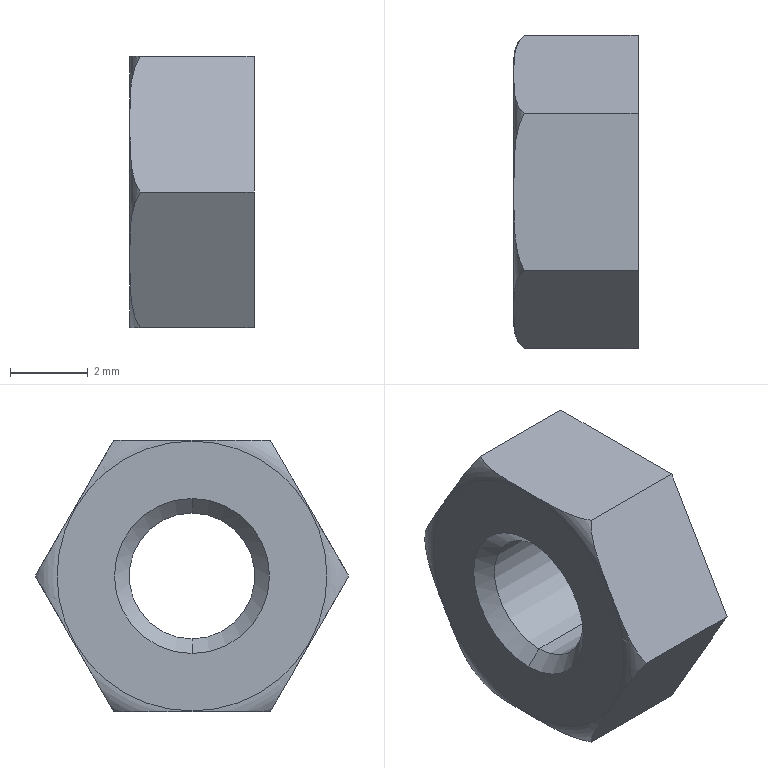Part | SolidWorks | features RefAxis 3, 3DProfileFeature 1, ICE 1, RevCut 1, Revolution 1 | 1 solid | 16 faces | box 3.2 x 8.083 x 7 mm | volume 107.662 mm3 | plane 8 | cone 4 | cylinder 2 | torus 2 | commonest cylinder face diameters 3.242 x2
STEP:
#1=CARTESIAN_POINT('',(1.221,0.,-1.621));
#2=VERTEX_POINT('',#1);
#3=CARTESIAN_POINT('',(1.221,0.,1.621));
#4=VERTEX_POINT('',#3);
#5=CARTESIAN_POINT('',(1.221,0.,0.));
#6=DIRECTION('',(-1.,0.,0.));
#7=DIRECTION('',(0.,0.,1.));
#8=AXIS2_PLACEMENT_3D('',#5,#6,#7);
#9=CIRCLE('',#8,1.621);
#10=EDGE_CURVE('',#2,#4,#9,.T.);
#11=ORIENTED_EDGE('',*,*,#10,.T.);
#12=CARTESIAN_POINT('',(1.6,0.,2.));
#13=VERTEX_POINT('',#12);
#14=CARTESIAN_POINT('',(1.6,0.,2.));
#15=DIRECTION('',(0.7071,0.,0.7071));
#16=VECTOR('',#15,1000.);
#17=LINE('',#14,#16);
#18=EDGE_CURVE('',#4,#13,#17,.T.);
#19=ORIENTED_EDGE('',*,*,#18,.T.);
#20=CARTESIAN_POINT('',(1.6,0.,-2.));
#21=VERTEX_POINT('',#20);
#22=CARTESIAN_POINT('',(1.6,0.,0.));
#23=DIRECTION('',(-1.,0.,0.));
#24=DIRECTION('',(0.,0.,1.));
#25=AXIS2_PLACEMENT_3D('',#22,#23,#24);
#26=CIRCLE('',#25,2.);
#27=EDGE_CURVE('',#21,#13,#26,.T.);
#28=ORIENTED_EDGE('',*,*,#27,.F.);
#29=CARTESIAN_POINT('',(1.6,0.,-2.));
#30=DIRECTION('',(0.7071,0.,-0.7071));
#31=VECTOR('',#30,1000.);
#32=LINE('',#29,#31);
#33=EDGE_CURVE('',#2,#21,#32,.T.);
#34=ORIENTED_EDGE('',*,*,#33,.F.);
#35=EDGE_LOOP('',(#11,#19,#28,#34));
#36=FACE_OUTER_BOUND('',#35,.T.);
#37=CARTESIAN_POINT('',(1.6,0.,0.));
#38=DIRECTION('',(1.,0.,0.));
#39=DIRECTION('',(0.,0.,-1.));
#40=AXIS2_PLACEMENT_3D('',#37,#38,#39);
#41=CONICAL_SURFACE('',#40,2.,0.7854);
#42=ADVANCED_FACE('',(#36),#41,.F.);
#43=ORIENTED_EDGE('',*,*,#10,.F.);
#44=CARTESIAN_POINT('',(-1.221,0.,-1.621));
#45=VERTEX_POINT('',#44);
#46=CARTESIAN_POINT('',(1.6,0.,-1.621));
#47=DIRECTION('',(-1.,0.,0.));
#48=VECTOR('',#47,1000.);
#49=LINE('',#46,#48);
#50=EDGE_CURVE('',#2,#45,#49,.T.);
#51=ORIENTED_EDGE('',*,*,#50,.T.);
#52=CARTESIAN_POINT('',(-1.221,0.,1.621));
#53=VERTEX_POINT('',#52);
#54=CARTESIAN_POINT('',(-1.221,0.,0.));
#55=DIRECTION('',(-1.,0.,0.));
#56=DIRECTION('',(0.,0.,1.));
#57=AXIS2_PLACEMENT_3D('',#54,#55,#56);
#58=CIRCLE('',#57,1.621);
#59=EDGE_CURVE('',#45,#53,#58,.T.);
#60=ORIENTED_EDGE('',*,*,#59,.T.);
#61=CARTESIAN_POINT('',(1.6,0.,1.621));
#62=DIRECTION('',(-1.,0.,0.));
#63=VECTOR('',#62,1000.);
#64=LINE('',#61,#63);
#65=EDGE_CURVE('',#4,#53,#64,.T.);
#66=ORIENTED_EDGE('',*,*,#65,.F.);
#67=EDGE_LOOP('',(#43,#51,#60,#66));
#68=FACE_OUTER_BOUND('',#67,.T.);
#69=CARTESIAN_POINT('',(1.6,0.,0.));
#70=DIRECTION('',(-1.,0.,0.));
#71=DIRECTION('',(0.,0.,1.));
#72=AXIS2_PLACEMENT_3D('',#69,#70,#71);
#73=CYLINDRICAL_SURFACE('',#72,1.621);
#74=ADVANCED_FACE('',(#68),#73,.F.);
#75=ORIENTED_EDGE('',*,*,#59,.F.);
#76=CARTESIAN_POINT('',(-1.6,0.,-2.));
#77=VERTEX_POINT('',#76);
#78=CARTESIAN_POINT('',(-1.221,0.,-1.621));
#79=DIRECTION('',(-0.7071,0.,-0.7071));
#80=VECTOR('',#79,1000.);
#81=LINE('',#78,#80);
#82=EDGE_CURVE('',#45,#77,#81,.T.);
#83=ORIENTED_EDGE('',*,*,#82,.T.);
#84=CARTESIAN_POINT('',(-1.6,0.,2.));
#85=VERTEX_POINT('',#84);
#86=CARTESIAN_POINT('',(-1.6,0.,0.));
#87=DIRECTION('',(-1.,0.,0.));
#88=DIRECTION('',(0.,0.,1.));
#89=AXIS2_PLACEMENT_3D('',#86,#87,#88);
#90=CIRCLE('',#89,2.);
#91=EDGE_CURVE('',#77,#85,#90,.T.);
#92=ORIENTED_EDGE('',*,*,#91,.T.);
#93=CARTESIAN_POINT('',(-1.221,0.,1.621));
#94=DIRECTION('',(-0.7071,0.,0.7071));
#95=VECTOR('',#94,1000.);
#96=LINE('',#93,#95);
#97=EDGE_CURVE('',#53,#85,#96,.T.);
#98=ORIENTED_EDGE('',*,*,#97,.F.);
#99=EDGE_LOOP('',(#75,#83,#92,#98));
#100=FACE_OUTER_BOUND('',#99,.T.);
#101=CARTESIAN_POINT('',(-1.221,0.,0.));
#102=DIRECTION('',(-1.,0.,0.));
#103=DIRECTION('',(0.,0.,1.));
#104=AXIS2_PLACEMENT_3D('',#101,#102,#103);
#105=CONICAL_SURFACE('',#104,1.621,0.7854);
#106=ADVANCED_FACE('',(#100),#105,.F.);
#107=CARTESIAN_POINT('',(-1.6,0.,-3.5));
#108=VERTEX_POINT('',#107);
#109=CARTESIAN_POINT('',(-1.331,2.021,-3.5));
#110=VERTEX_POINT('',#109);
#111=CARTESIAN_POINT('',(-1.6,0.,-3.5));
#112=CARTESIAN_POINT('',(-1.6,0.3431,-3.5));
#113=CARTESIAN_POINT('',(-1.603,0.6864,-3.5));
#114=CARTESIAN_POINT('',(-1.569,1.2,-3.5));
#115=CARTESIAN_POINT('',(-1.549,1.371,-3.5));
#116=CARTESIAN_POINT('',(-1.494,1.624,-3.5));
#117=CARTESIAN_POINT('',(-1.472,1.706,-3.5));
#118=CARTESIAN_POINT('',(-1.413,1.868,-3.5));
#119=CARTESIAN_POINT('',(-1.376,1.948,-3.5));
#120=CARTESIAN_POINT('',(-1.331,2.021,-3.5));
#121=B_SPLINE_CURVE_WITH_KNOTS('',3,(#111,#112,#113,#114,#115,#116,#117,#118,#119,#120),.UNSPECIFIED.,.F.,.F.,(4,2,2,2,4),(0.,0.001028,0.001542,0.001799,0.002057),.UNSPECIFIED.);
#122=EDGE_CURVE('',#108,#110,#121,.T.);
#123=ORIENTED_EDGE('',*,*,#122,.F.);
#124=CARTESIAN_POINT('',(-1.6,0.,-3.48));
#125=VERTEX_POINT('',#124);
#126=CARTESIAN_POINT('',(-0.88,0.,-3.48));
#127=DIRECTION('',(0.,1.,0.));
#128=DIRECTION('',(0.,0.,1.));
#129=AXIS2_PLACEMENT_3D('',#126,#127,#128);
#130=CIRCLE('',#129,0.72);
#131=EDGE_CURVE('',#108,#125,#130,.T.);
#132=ORIENTED_EDGE('',*,*,#131,.T.);
#133=CARTESIAN_POINT('',(-1.6,0.,3.48));
#134=VERTEX_POINT('',#133);
#135=CARTESIAN_POINT('',(-1.6,0.,0.));
#136=DIRECTION('',(-1.,0.,0.));
#137=DIRECTION('',(0.,0.,1.));
#138=AXIS2_PLACEMENT_3D('',#135,#136,#137);
#139=CIRCLE('',#138,3.48);
#140=EDGE_CURVE('',#134,#125,#139,.T.);
#141=ORIENTED_EDGE('',*,*,#140,.F.);
#142=CARTESIAN_POINT('',(-1.6,0.,3.5));
#143=VERTEX_POINT('',#142);
#144=CARTESIAN_POINT('',(-0.88,0.,3.48));
#145=DIRECTION('',(0.,-1.,0.));
#146=DIRECTION('',(0.,0.,-1.));
#147=AXIS2_PLACEMENT_3D('',#144,#145,#146);
#148=CIRCLE('',#147,0.72);
#149=EDGE_CURVE('',#143,#134,#148,.T.);
#150=ORIENTED_EDGE('',*,*,#149,.F.);
#151=CARTESIAN_POINT('',(-1.331,2.021,3.5));
#152=VERTEX_POINT('',#151);
#153=CARTESIAN_POINT('',(-1.331,2.021,3.5));
#154=CARTESIAN_POINT('',(-1.422,1.874,3.5));
#155=CARTESIAN_POINT('',(-1.476,1.706,3.5));
#156=CARTESIAN_POINT('',(-1.549,1.372,3.5));
#157=CARTESIAN_POINT('',(-1.568,1.202,3.5));
#158=CARTESIAN_POINT('',(-1.592,0.8597,3.5));
#159=CARTESIAN_POINT('',(-1.596,0.6875,3.5));
#160=CARTESIAN_POINT('',(-1.6,0.3438,3.5));
#161=CARTESIAN_POINT('',(-1.6,0.1724,3.5));
#162=CARTESIAN_POINT('',(-1.6,0.,3.5));
#163=B_SPLINE_CURVE_WITH_KNOTS('',3,(#153,#154,#155,#156,#157,#158,#159,#160,#161,#162),.UNSPECIFIED.,.F.,.F.,(4,2,2,2,4),(0.008439,0.008956,0.009473,0.009989,0.01051),.UNSPECIFIED.);
#164=EDGE_CURVE('',#152,#143,#163,.T.);
#165=ORIENTED_EDGE('',*,*,#164,.F.);
#166=CARTESIAN_POINT('',(-1.331,4.041,0.));
#167=VERTEX_POINT('',#166);
#168=CARTESIAN_POINT('',(-1.331,4.041,0.));
#169=CARTESIAN_POINT('',(-1.424,3.967,0.1292));
#170=CARTESIAN_POINT('',(-1.477,3.884,0.2733));
#171=CARTESIAN_POINT('',(-1.55,3.714,0.5673));
#172=CARTESIAN_POINT('',(-1.569,3.629,0.7151));
#173=CARTESIAN_POINT('',(-1.603,3.372,1.159));
#174=CARTESIAN_POINT('',(-1.6,3.2,1.457));
#175=CARTESIAN_POINT('',(-1.6,2.857,2.051));
#176=CARTESIAN_POINT('',(-1.603,2.686,2.348));
#177=CARTESIAN_POINT('',(-1.568,2.429,2.793));
#178=CARTESIAN_POINT('',(-1.549,2.343,2.941));
#179=CARTESIAN_POINT('',(-1.475,2.176,3.231));
#180=CARTESIAN_POINT('',(-1.423,2.095,3.372));
#181=CARTESIAN_POINT('',(-1.331,2.021,3.5));
#182=B_SPLINE_CURVE_WITH_KNOTS('',3,(#168,#169,#170,#171,#172,#173,#174,#175,#176,#177,#178,#179,#180,#181),.UNSPECIFIED.,.F.,.F.,(4,2,2,2,2,2,4),(0.000000268,0.0005191,0.001038,0.002076,0.003113,0.003632,0.004151),.UNSPECIFIED.);
#183=EDGE_CURVE('',#167,#152,#182,.T.);
#184=ORIENTED_EDGE('',*,*,#183,.F.);
#185=CARTESIAN_POINT('',(-1.331,2.021,-3.5));
#186=CARTESIAN_POINT('',(-1.424,2.095,-3.371));
#187=CARTESIAN_POINT('',(-1.477,2.179,-3.227));
#188=CARTESIAN_POINT('',(-1.55,2.348,-2.933));
#189=CARTESIAN_POINT('',(-1.569,2.434,-2.785));
#190=CARTESIAN_POINT('',(-1.603,2.69,-2.341));
#191=CARTESIAN_POINT('',(-1.6,2.862,-2.043));
#192=CARTESIAN_POINT('',(-1.6,3.205,-1.449));
#193=CARTESIAN_POINT('',(-1.603,3.377,-1.152));
#194=CARTESIAN_POINT('',(-1.568,3.633,-0.7074));
#195=CARTESIAN_POINT('',(-1.549,3.719,-0.5586));
#196=CARTESIAN_POINT('',(-1.475,3.886,-0.2687));
#197=CARTESIAN_POINT('',(-1.423,3.967,-0.1283));
#198=CARTESIAN_POINT('',(-1.331,4.041,0.));
#199=B_SPLINE_CURVE_WITH_KNOTS('',3,(#185,#186,#187,#188,#189,#190,#191,#192,#193,#194,#195,#196,#197,#198),.UNSPECIFIED.,.F.,.F.,(4,2,2,2,2,2,4),(0.000000268,0.0005191,0.001038,0.002076,0.003113,0.003632,0.004151),.UNSPECIFIED.);
#200=EDGE_CURVE('',#110,#167,#199,.T.);
#201=ORIENTED_EDGE('',*,*,#200,.F.);
#202=EDGE_LOOP('',(#123,#132,#141,#150,#165,#184,#201));
#203=FACE_OUTER_BOUND('',#202,.T.);
#204=CARTESIAN_POINT('',(-0.88,0.,0.));
#205=DIRECTION('',(-1.,0.,0.));
#206=DIRECTION('',(0.,0.,1.));
#207=AXIS2_PLACEMENT_3D('',#204,#205,#206);
#208=TOROIDAL_SURFACE('',#207,3.48,0.72);
#209=ADVANCED_FACE('',(#203),#208,.T.);
#210=ORIENTED_EDGE('',*,*,#27,.T.);
#211=CARTESIAN_POINT('',(1.6,0.,0.));
#212=DIRECTION('',(-1.,0.,0.));
#213=DIRECTION('',(0.,0.,1.));
#214=AXIS2_PLACEMENT_3D('',#211,#212,#213);
#215=CIRCLE('',#214,2.);
#216=EDGE_CURVE('',#13,#21,#215,.T.);
#217=ORIENTED_EDGE('',*,*,#216,.T.);
#218=EDGE_LOOP('',(#210,#217));
#219=FACE_BOUND('',#218,.T.);
#220=CARTESIAN_POINT('',(1.6,4.041,0.));
#221=VERTEX_POINT('',#220);
#222=CARTESIAN_POINT('',(1.6,2.021,3.5));
#223=VERTEX_POINT('',#222);
#224=CARTESIAN_POINT('',(1.6,4.041,0.));
#225=DIRECTION('',(0.,-0.5,0.866));
#226=VECTOR('',#225,1000.);
#227=LINE('',#224,#226);
#228=EDGE_CURVE('',#221,#223,#227,.T.);
#229=ORIENTED_EDGE('',*,*,#228,.T.);
#230=CARTESIAN_POINT('',(1.6,-2.021,3.5));
#231=VERTEX_POINT('',#230);
#232=CARTESIAN_POINT('',(1.6,2.021,3.5));
#233=DIRECTION('',(0.,-1.,0.));
#234=VECTOR('',#233,1000.);
#235=LINE('',#232,#234);
#236=EDGE_CURVE('',#223,#231,#235,.T.);
#237=ORIENTED_EDGE('',*,*,#236,.T.);
#238=CARTESIAN_POINT('',(1.6,-4.041,0.));
#239=VERTEX_POINT('',#238);
#240=CARTESIAN_POINT('',(1.6,-2.021,3.5));
#241=DIRECTION('',(0.,-0.5,-0.866));
#242=VECTOR('',#241,1000.);
#243=LINE('',#240,#242);
#244=EDGE_CURVE('',#231,#239,#243,.T.);
#245=ORIENTED_EDGE('',*,*,#244,.T.);
#246=CARTESIAN_POINT('',(1.6,-2.021,-3.5));
#247=VERTEX_POINT('',#246);
#248=CARTESIAN_POINT('',(1.6,-4.041,0.));
#249=DIRECTION('',(0.,0.5,-0.866));
#250=VECTOR('',#249,1000.);
#251=LINE('',#248,#250);
#252=EDGE_CURVE('',#239,#247,#251,.T.);
#253=ORIENTED_EDGE('',*,*,#252,.T.);
#254=CARTESIAN_POINT('',(1.6,2.021,-3.5));
#255=VERTEX_POINT('',#254);
#256=CARTESIAN_POINT('',(1.6,-2.021,-3.5));
#257=DIRECTION('',(0.,1.,0.));
#258=VECTOR('',#257,1000.);
#259=LINE('',#256,#258);
#260=EDGE_CURVE('',#247,#255,#259,.T.);
#261=ORIENTED_EDGE('',*,*,#260,.T.);
#262=CARTESIAN_POINT('',(1.6,2.021,-3.5));
#263=DIRECTION('',(0.,0.5,0.866));
#264=VECTOR('',#263,1000.);
#265=LINE('',#262,#264);
#266=EDGE_CURVE('',#255,#221,#265,.T.);
#267=ORIENTED_EDGE('',*,*,#266,.T.);
#268=EDGE_LOOP('',(#229,#237,#245,#253,#261,#267));
#269=FACE_OUTER_BOUND('',#268,.T.);
#270=CARTESIAN_POINT('',(1.6,4.2,0.));
#271=DIRECTION('',(-1.,0.,0.));
#272=DIRECTION('',(0.,0.,1.));
#273=AXIS2_PLACEMENT_3D('',#270,#271,#272);
#274=PLANE('',#273);
#275=ADVANCED_FACE('',(#219,#269),#274,.F.);
#276=ORIENTED_EDGE('',*,*,#131,.F.);
#277=CARTESIAN_POINT('',(-1.331,-2.021,-3.5));
#278=VERTEX_POINT('',#277);
#279=CARTESIAN_POINT('',(-1.331,-2.021,-3.5));
#280=CARTESIAN_POINT('',(-1.422,-1.874,-3.5));
#281=CARTESIAN_POINT('',(-1.476,-1.706,-3.5));
#282=CARTESIAN_POINT('',(-1.549,-1.372,-3.5));
#283=CARTESIAN_POINT('',(-1.568,-1.202,-3.5));
#284=CARTESIAN_POINT('',(-1.592,-0.8597,-3.5));
#285=CARTESIAN_POINT('',(-1.596,-0.6875,-3.5));
#286=CARTESIAN_POINT('',(-1.6,-0.3438,-3.5));
#287=CARTESIAN_POINT('',(-1.6,-0.1724,-3.5));
#288=CARTESIAN_POINT('',(-1.6,0.,-3.5));
#289=B_SPLINE_CURVE_WITH_KNOTS('',3,(#279,#280,#281,#282,#283,#284,#285,#286,#287,#288),.UNSPECIFIED.,.F.,.F.,(4,2,2,2,4),(0.008439,0.008956,0.009473,0.009989,0.01051),.UNSPECIFIED.);
#290=EDGE_CURVE('',#278,#108,#289,.T.);
#291=ORIENTED_EDGE('',*,*,#290,.F.);
#292=CARTESIAN_POINT('',(-1.331,-4.041,0.));
#293=VERTEX_POINT('',#292);
#294=CARTESIAN_POINT('',(-1.331,-4.041,0.));
#295=CARTESIAN_POINT('',(-1.424,-3.967,-0.1292));
#296=CARTESIAN_POINT('',(-1.477,-3.884,-0.2733));
#297=CARTESIAN_POINT('',(-1.55,-3.714,-0.5673));
#298=CARTESIAN_POINT('',(-1.569,-3.629,-0.7151));
#299=CARTESIAN_POINT('',(-1.603,-3.372,-1.159));
#300=CARTESIAN_POINT('',(-1.6,-3.2,-1.457));
#301=CARTESIAN_POINT('',(-1.6,-2.857,-2.051));
#302=CARTESIAN_POINT('',(-1.603,-2.686,-2.348));
#303=CARTESIAN_POINT('',(-1.568,-2.429,-2.793));
#304=CARTESIAN_POINT('',(-1.549,-2.343,-2.941));
#305=CARTESIAN_POINT('',(-1.475,-2.176,-3.231));
#306=CARTESIAN_POINT('',(-1.423,-2.095,-3.372));
#307=CARTESIAN_POINT('',(-1.331,-2.021,-3.5));
#308=B_SPLINE_CURVE_WITH_KNOTS('',3,(#294,#295,#296,#297,#298,#299,#300,#301,#302,#303,#304,#305,#306,#307),.UNSPECIFIED.,.F.,.F.,(4,2,2,2,2,2,4),(0.000000268,0.0005191,0.001038,0.002076,0.003113,0.003632,0.004151),.UNSPECIFIED.);
#309=EDGE_CURVE('',#293,#278,#308,.T.);
#310=ORIENTED_EDGE('',*,*,#309,.F.);
#311=CARTESIAN_POINT('',(-1.331,-2.021,3.5));
#312=VERTEX_POINT('',#311);
#313=CARTESIAN_POINT('',(-1.331,-2.021,3.5));
#314=CARTESIAN_POINT('',(-1.424,-2.095,3.371));
#315=CARTESIAN_POINT('',(-1.477,-2.179,3.227));
#316=CARTESIAN_POINT('',(-1.55,-2.348,2.933));
#317=CARTESIAN_POINT('',(-1.569,-2.434,2.785));
#318=CARTESIAN_POINT('',(-1.603,-2.69,2.341));
#319=CARTESIAN_POINT('',(-1.6,-2.862,2.043));
#320=CARTESIAN_POINT('',(-1.6,-3.205,1.449));
#321=CARTESIAN_POINT('',(-1.603,-3.377,1.152));
#322=CARTESIAN_POINT('',(-1.568,-3.633,0.7074));
#323=CARTESIAN_POINT('',(-1.549,-3.719,0.5586));
#324=CARTESIAN_POINT('',(-1.475,-3.886,0.2687));
#325=CARTESIAN_POINT('',(-1.423,-3.967,0.1283));
#326=CARTESIAN_POINT('',(-1.331,-4.041,0.));
#327=B_SPLINE_CURVE_WITH_KNOTS('',3,(#313,#314,#315,#316,#317,#318,#319,#320,#321,#322,#323,#324,#325,#326),.UNSPECIFIED.,.F.,.F.,(4,2,2,2,2,2,4),(0.000000268,0.0005191,0.001038,0.002076,0.003113,0.003632,0.004151),.UNSPECIFIED.);
#328=EDGE_CURVE('',#312,#293,#327,.T.);
#329=ORIENTED_EDGE('',*,*,#328,.F.);
#330=CARTESIAN_POINT('',(-1.6,0.,3.5));
#331=CARTESIAN_POINT('',(-1.6,-0.3431,3.5));
#332=CARTESIAN_POINT('',(-1.603,-0.6864,3.5));
#333=CARTESIAN_POINT('',(-1.569,-1.2,3.5));
#334=CARTESIAN_POINT('',(-1.549,-1.371,3.5));
#335=CARTESIAN_POINT('',(-1.494,-1.624,3.5));
#336=CARTESIAN_POINT('',(-1.472,-1.706,3.5));
#337=CARTESIAN_POINT('',(-1.413,-1.868,3.5));
#338=CARTESIAN_POINT('',(-1.376,-1.948,3.5));
#339=CARTESIAN_POINT('',(-1.331,-2.021,3.5));
#340=B_SPLINE_CURVE_WITH_KNOTS('',3,(#330,#331,#332,#333,#334,#335,#336,#337,#338,#339),.UNSPECIFIED.,.F.,.F.,(4,2,2,2,4),(0.,0.001028,0.001542,0.001799,0.002057),.UNSPECIFIED.);
#341=EDGE_CURVE('',#143,#312,#340,.T.);
#342=ORIENTED_EDGE('',*,*,#341,.F.);
#343=ORIENTED_EDGE('',*,*,#149,.T.);
#344=CARTESIAN_POINT('',(-1.6,0.,0.));
#345=DIRECTION('',(-1.,0.,0.));
#346=DIRECTION('',(0.,0.,1.));
#347=AXIS2_PLACEMENT_3D('',#344,#345,#346);
#348=CIRCLE('',#347,3.48);
#349=EDGE_CURVE('',#125,#134,#348,.T.);
#350=ORIENTED_EDGE('',*,*,#349,.F.);
#351=EDGE_LOOP('',(#276,#291,#310,#329,#342,#343,#350));
#352=FACE_OUTER_BOUND('',#351,.T.);
#353=CARTESIAN_POINT('',(-0.88,0.,0.));
#354=DIRECTION('',(-1.,0.,0.));
#355=DIRECTION('',(0.,0.,1.));
#356=AXIS2_PLACEMENT_3D('',#353,#354,#355);
#357=TOROIDAL_SURFACE('',#356,3.48,0.72);
#358=ADVANCED_FACE('',(#352),#357,.T.);
#359=ORIENTED_EDGE('',*,*,#140,.T.);
#360=ORIENTED_EDGE('',*,*,#349,.T.);
#361=EDGE_LOOP('',(#359,#360));
#362=FACE_OUTER_BOUND('',#361,.T.);
#363=CARTESIAN_POINT('',(-1.6,0.,0.));
#364=DIRECTION('',(-1.,0.,0.));
#365=DIRECTION('',(0.,0.,1.));
#366=AXIS2_PLACEMENT_3D('',#363,#364,#365);
#367=CIRCLE('',#366,2.);
#368=EDGE_CURVE('',#85,#77,#367,.T.);
#369=ORIENTED_EDGE('',*,*,#368,.F.);
#370=ORIENTED_EDGE('',*,*,#91,.F.);
#371=EDGE_LOOP('',(#369,#370));
#372=FACE_BOUND('',#371,.T.);
#373=CARTESIAN_POINT('',(-1.6,0.,0.));
#374=DIRECTION('',(1.,0.,0.));
#375=DIRECTION('',(0.,0.,-1.));
#376=AXIS2_PLACEMENT_3D('',#373,#374,#375);
#377=PLANE('',#376);
#378=ADVANCED_FACE('',(#362,#372),#377,.F.);
#379=ORIENTED_EDGE('',*,*,#82,.F.);
#380=CARTESIAN_POINT('',(-1.221,0.,0.));
#381=DIRECTION('',(-1.,0.,0.));
#382=DIRECTION('',(0.,0.,1.));
#383=AXIS2_PLACEMENT_3D('',#380,#381,#382);
#384=CIRCLE('',#383,1.621);
#385=EDGE_CURVE('',#53,#45,#384,.T.);
#386=ORIENTED_EDGE('',*,*,#385,.F.);
#387=ORIENTED_EDGE('',*,*,#97,.T.);
#388=ORIENTED_EDGE('',*,*,#368,.T.);
#389=EDGE_LOOP('',(#379,#386,#387,#388));
#390=FACE_OUTER_BOUND('',#389,.T.);
#391=CARTESIAN_POINT('',(-1.221,0.,0.));
#392=DIRECTION('',(-1.,0.,0.));
#393=DIRECTION('',(0.,0.,1.));
#394=AXIS2_PLACEMENT_3D('',#391,#392,#393);
#395=CONICAL_SURFACE('',#394,1.621,0.7854);
#396=ADVANCED_FACE('',(#390),#395,.F.);
#397=ORIENTED_EDGE('',*,*,#50,.F.);
#398=CARTESIAN_POINT('',(1.221,0.,0.));
#399=DIRECTION('',(-1.,0.,0.));
#400=DIRECTION('',(0.,0.,1.));
#401=AXIS2_PLACEMENT_3D('',#398,#399,#400);
#402=CIRCLE('',#401,1.621);
#403=EDGE_CURVE('',#4,#2,#402,.T.);
#404=ORIENTED_EDGE('',*,*,#403,.F.);
#405=ORIENTED_EDGE('',*,*,#65,.T.);
#406=ORIENTED_EDGE('',*,*,#385,.T.);
#407=EDGE_LOOP('',(#397,#404,#405,#406));
#408=FACE_OUTER_BOUND('',#407,.T.);
#409=CARTESIAN_POINT('',(1.6,0.,0.));
#410=DIRECTION('',(-1.,0.,0.));
#411=DIRECTION('',(0.,0.,1.));
#412=AXIS2_PLACEMENT_3D('',#409,#410,#411);
#413=CYLINDRICAL_SURFACE('',#412,1.621);
#414=ADVANCED_FACE('',(#408),#413,.F.);
#415=ORIENTED_EDGE('',*,*,#18,.F.);
#416=ORIENTED_EDGE('',*,*,#403,.T.);
#417=ORIENTED_EDGE('',*,*,#33,.T.);
#418=ORIENTED_EDGE('',*,*,#216,.F.);
#419=EDGE_LOOP('',(#415,#416,#417,#418));
#420=FACE_OUTER_BOUND('',#419,.T.);
#421=CARTESIAN_POINT('',(1.6,0.,0.));
#422=DIRECTION('',(1.,0.,0.));
#423=DIRECTION('',(0.,0.,-1.));
#424=AXIS2_PLACEMENT_3D('',#421,#422,#423);
#425=CONICAL_SURFACE('',#424,2.,0.7854);
#426=ADVANCED_FACE('',(#420),#425,.F.);
#427=ORIENTED_EDGE('',*,*,#183,.T.);
#428=CARTESIAN_POINT('',(-1.6,2.021,3.5));
#429=DIRECTION('',(1.,0.,0.));
#430=VECTOR('',#429,1000.);
#431=LINE('',#428,#430);
#432=EDGE_CURVE('',#152,#223,#431,.T.);
#433=ORIENTED_EDGE('',*,*,#432,.T.);
#434=ORIENTED_EDGE('',*,*,#228,.F.);
#435=CARTESIAN_POINT('',(-1.6,4.041,0.));
#436=DIRECTION('',(1.,0.,0.));
#437=VECTOR('',#436,1000.);
#438=LINE('',#435,#437);
#439=EDGE_CURVE('',#167,#221,#438,.T.);
#440=ORIENTED_EDGE('',*,*,#439,.F.);
#441=EDGE_LOOP('',(#427,#433,#434,#440));
#442=FACE_OUTER_BOUND('',#441,.T.);
#443=CARTESIAN_POINT('',(-1.6,4.041,0.));
#444=DIRECTION('',(0.,0.866,0.5));
#445=DIRECTION('',(0.,-0.5,0.866));
#446=AXIS2_PLACEMENT_3D('',#443,#444,#445);
#447=PLANE('',#446);
#448=ADVANCED_FACE('',(#442),#447,.T.);
#449=ORIENTED_EDGE('',*,*,#200,.T.);
#450=ORIENTED_EDGE('',*,*,#439,.T.);
#451=ORIENTED_EDGE('',*,*,#266,.F.);
#452=CARTESIAN_POINT('',(-1.6,2.021,-3.5));
#453=DIRECTION('',(1.,0.,0.));
#454=VECTOR('',#453,1000.);
#455=LINE('',#452,#454);
#456=EDGE_CURVE('',#110,#255,#455,.T.);
#457=ORIENTED_EDGE('',*,*,#456,.F.);
#458=EDGE_LOOP('',(#449,#450,#451,#457));
#459=FACE_OUTER_BOUND('',#458,.T.);
#460=CARTESIAN_POINT('',(-1.6,2.021,-3.5));
#461=DIRECTION('',(0.,0.866,-0.5));
#462=DIRECTION('',(0.,0.5,0.866));
#463=AXIS2_PLACEMENT_3D('',#460,#461,#462);
#464=PLANE('',#463);
#465=ADVANCED_FACE('',(#459),#464,.T.);
#466=ORIENTED_EDGE('',*,*,#290,.T.);
#467=ORIENTED_EDGE('',*,*,#122,.T.);
#468=ORIENTED_EDGE('',*,*,#456,.T.);
#469=ORIENTED_EDGE('',*,*,#260,.F.);
#470=CARTESIAN_POINT('',(-1.6,-2.021,-3.5));
#471=DIRECTION('',(1.,0.,0.));
#472=VECTOR('',#471,1000.);
#473=LINE('',#470,#472);
#474=EDGE_CURVE('',#278,#247,#473,.T.);
#475=ORIENTED_EDGE('',*,*,#474,.F.);
#476=EDGE_LOOP('',(#466,#467,#468,#469,#475));
#477=FACE_OUTER_BOUND('',#476,.T.);
#478=CARTESIAN_POINT('',(-1.6,-2.021,-3.5));
#479=DIRECTION('',(0.,0.,-1.));
#480=DIRECTION('',(-1.,0.,0.));
#481=AXIS2_PLACEMENT_3D('',#478,#479,#480);
#482=PLANE('',#481);
#483=ADVANCED_FACE('',(#477),#482,.T.);
#484=ORIENTED_EDGE('',*,*,#309,.T.);
#485=ORIENTED_EDGE('',*,*,#474,.T.);
#486=ORIENTED_EDGE('',*,*,#252,.F.);
#487=CARTESIAN_POINT('',(-1.6,-4.041,0.));
#488=DIRECTION('',(1.,0.,0.));
#489=VECTOR('',#488,1000.);
#490=LINE('',#487,#489);
#491=EDGE_CURVE('',#293,#239,#490,.T.);
#492=ORIENTED_EDGE('',*,*,#491,.F.);
#493=EDGE_LOOP('',(#484,#485,#486,#492));
#494=FACE_OUTER_BOUND('',#493,.T.);
#495=CARTESIAN_POINT('',(-1.6,-4.041,0.));
#496=DIRECTION('',(0.,-0.866,-0.5));
#497=DIRECTION('',(0.,0.5,-0.866));
#498=AXIS2_PLACEMENT_3D('',#495,#496,#497);
#499=PLANE('',#498);
#500=ADVANCED_FACE('',(#494),#499,.T.);
#501=ORIENTED_EDGE('',*,*,#328,.T.);
#502=ORIENTED_EDGE('',*,*,#491,.T.);
#503=ORIENTED_EDGE('',*,*,#244,.F.);
#504=CARTESIAN_POINT('',(-1.6,-2.021,3.5));
#505=DIRECTION('',(1.,0.,0.));
#506=VECTOR('',#505,1000.);
#507=LINE('',#504,#506);
#508=EDGE_CURVE('',#312,#231,#507,.T.);
#509=ORIENTED_EDGE('',*,*,#508,.F.);
#510=EDGE_LOOP('',(#501,#502,#503,#509));
#511=FACE_OUTER_BOUND('',#510,.T.);
#512=CARTESIAN_POINT('',(-1.6,-2.021,3.5));
#513=DIRECTION('',(0.,-0.866,0.5));
#514=DIRECTION('',(0.,-0.5,-0.866));
#515=AXIS2_PLACEMENT_3D('',#512,#513,#514);
#516=PLANE('',#515);
#517=ADVANCED_FACE('',(#511),#516,.T.);
#518=ORIENTED_EDGE('',*,*,#164,.T.);
#519=ORIENTED_EDGE('',*,*,#341,.T.);
#520=ORIENTED_EDGE('',*,*,#508,.T.);
#521=ORIENTED_EDGE('',*,*,#236,.F.);
#522=ORIENTED_EDGE('',*,*,#432,.F.);
#523=EDGE_LOOP('',(#518,#519,#520,#521,#522));
#524=FACE_OUTER_BOUND('',#523,.T.);
#525=CARTESIAN_POINT('',(-1.6,2.021,3.5));
#526=DIRECTION('',(0.,0.,1.));
#527=DIRECTION('',(1.,0.,0.));
#528=AXIS2_PLACEMENT_3D('',#525,#526,#527);
#529=PLANE('',#528);
#530=ADVANCED_FACE('',(#524),#529,.T.);
#531=CLOSED_SHELL('',(#42,#74,#106,#209,#275,#358,#378,#396,#414,#426,#448,#465,#483,#500,#517,#530));
#532=MANIFOLD_SOLID_BREP('',#531);
#533=CARTESIAN_POINT('',(0.,0.,0.));
#534=DIRECTION('',(0.,0.,1.));
#535=DIRECTION('',(1.,0.,0.));
#536=AXIS2_PLACEMENT_3D('',#533,#534,#535);
#537=(LENGTH_UNIT()NAMED_UNIT(*)SI_UNIT(.MILLI.,.METRE.));
#538=UNCERTAINTY_MEASURE_WITH_UNIT(LENGTH_MEASURE(0.00001),#537,'','');
#539=(NAMED_UNIT(*)PLANE_ANGLE_UNIT()SI_UNIT($,.RADIAN.));
#540=(NAMED_UNIT(*)SI_UNIT($,.STERADIAN.)SOLID_ANGLE_UNIT());
#541=(GEOMETRIC_REPRESENTATION_CONTEXT(3)GLOBAL_UNCERTAINTY_ASSIGNED_CONTEXT((#538))GLOBAL_UNIT_ASSIGNED_CONTEXT((#537,#539,#540))REPRESENTATION_CONTEXT('',''));
#542=ADVANCED_BREP_SHAPE_REPRESENTATION('',(#532,#536),#541);